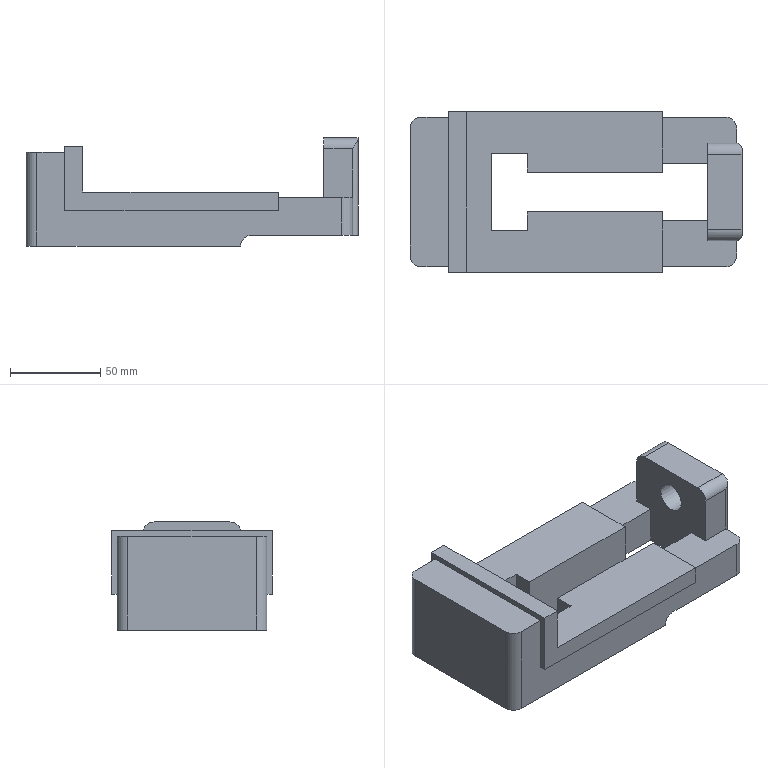Part | NX | features DATUM_CSYS 9, EXTRUDE 8, SKETCH 8, SIMPLE HOLE 6, SYMBOLIC_THREAD 6, HOLE PACKAGE 3, BLEND 1, CBORE_HOLE 1 | 1 solid | 65 faces | box 184 x 89 x 60 mm | volume 417123 mm3 | plane 35 | cylinder 18 | cone 12 | commonest cylinder face diameters 12 x8 6.8 x4 3.3 x2 6 x2 16 x1 27 x1